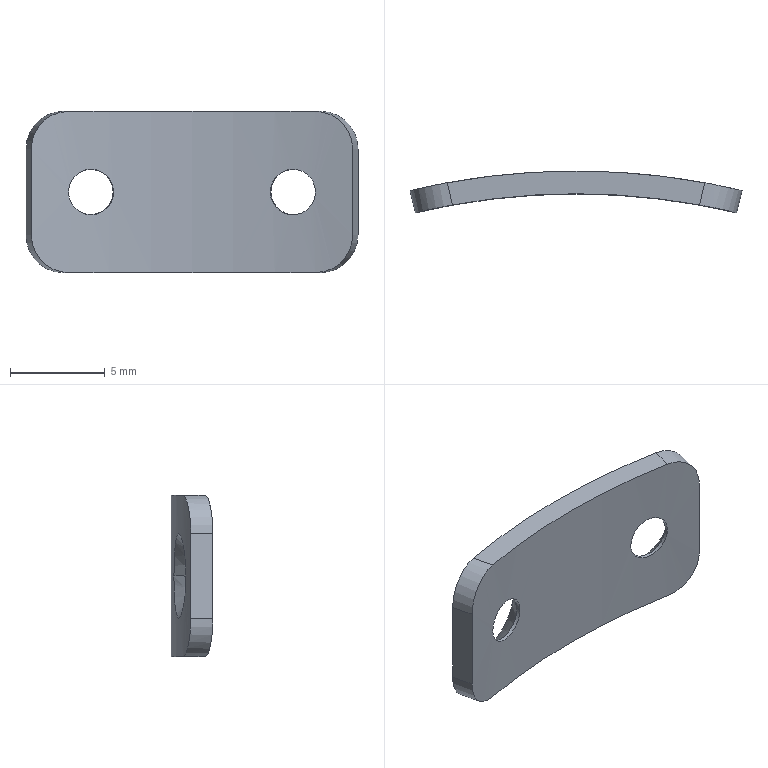Part | STEP file | 101000007768 | 1 solid | 18 faces | box 17.508 x 2.203 x 8.5 mm | volume 152.771 mm3 | cylinder 10 | cone 4 | plane 4 | commonest cylinder face diameters 2.4 x4 4 x4 72.6 x1 75 x1